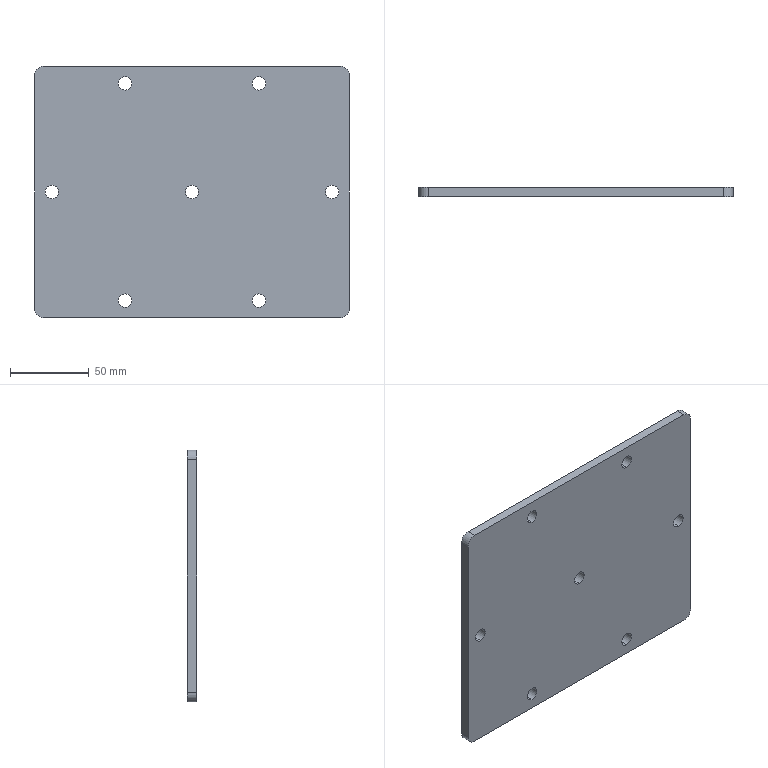Part | SolidWorks | features Extrusion 1, Fillet 1, HoleWzd 1 | 1 solid | 24 faces | box 200 x 6 x 160 mm | volume 189431 mm3 | cylinder 18 | plane 6 | commonest cylinder face diameters 8.5 x14 12 x4
STEP:
#1=CARTESIAN_POINT('',(0.,0.,-4.25));
#2=VERTEX_POINT('',#1);
#3=CARTESIAN_POINT('',(0.,0.,4.25));
#4=VERTEX_POINT('',#3);
#5=CARTESIAN_POINT('',(0.,0.,0.));
#6=DIRECTION('',(0.,1.,0.));
#7=DIRECTION('',(0.,0.,1.));
#8=AXIS2_PLACEMENT_3D('',#5,#6,#7);
#9=CIRCLE('',#8,4.25);
#10=EDGE_CURVE('',#2,#4,#9,.T.);
#11=ORIENTED_EDGE('',*,*,#10,.F.);
#12=CARTESIAN_POINT('',(0.,6.,-4.25));
#13=VERTEX_POINT('',#12);
#14=CARTESIAN_POINT('',(0.,6.,-4.25));
#15=DIRECTION('',(0.,1.,0.));
#16=VECTOR('',#15,1000.);
#17=LINE('',#14,#16);
#18=EDGE_CURVE('',#2,#13,#17,.T.);
#19=ORIENTED_EDGE('',*,*,#18,.T.);
#20=CARTESIAN_POINT('',(0.,6.,4.25));
#21=VERTEX_POINT('',#20);
#22=CARTESIAN_POINT('',(0.,6.,0.));
#23=DIRECTION('',(0.,1.,0.));
#24=DIRECTION('',(0.,0.,1.));
#25=AXIS2_PLACEMENT_3D('',#22,#23,#24);
#26=CIRCLE('',#25,4.25);
#27=EDGE_CURVE('',#13,#21,#26,.T.);
#28=ORIENTED_EDGE('',*,*,#27,.T.);
#29=CARTESIAN_POINT('',(0.,6.,4.25));
#30=DIRECTION('',(0.,1.,0.));
#31=VECTOR('',#30,1000.);
#32=LINE('',#29,#31);
#33=EDGE_CURVE('',#4,#21,#32,.T.);
#34=ORIENTED_EDGE('',*,*,#33,.F.);
#35=EDGE_LOOP('',(#11,#19,#28,#34));
#36=FACE_OUTER_BOUND('',#35,.T.);
#37=CARTESIAN_POINT('',(0.,6.,0.));
#38=DIRECTION('',(0.,1.,0.));
#39=DIRECTION('',(0.,0.,1.));
#40=AXIS2_PLACEMENT_3D('',#37,#38,#39);
#41=CYLINDRICAL_SURFACE('',#40,4.25);
#42=ADVANCED_FACE('',(#36),#41,.F.);
#43=CARTESIAN_POINT('',(42.5,0.,-73.25));
#44=VERTEX_POINT('',#43);
#45=CARTESIAN_POINT('',(42.5,0.,-64.75));
#46=VERTEX_POINT('',#45);
#47=CARTESIAN_POINT('',(42.5,0.,-69.));
#48=DIRECTION('',(0.,1.,0.));
#49=DIRECTION('',(0.,0.,1.));
#50=AXIS2_PLACEMENT_3D('',#47,#48,#49);
#51=CIRCLE('',#50,4.25);
#52=EDGE_CURVE('',#44,#46,#51,.T.);
#53=ORIENTED_EDGE('',*,*,#52,.F.);
#54=CARTESIAN_POINT('',(42.5,6.,-73.25));
#55=VERTEX_POINT('',#54);
#56=CARTESIAN_POINT('',(42.5,6.,-73.25));
#57=DIRECTION('',(0.,1.,0.));
#58=VECTOR('',#57,1000.);
#59=LINE('',#56,#58);
#60=EDGE_CURVE('',#44,#55,#59,.T.);
#61=ORIENTED_EDGE('',*,*,#60,.T.);
#62=CARTESIAN_POINT('',(42.5,6.,-64.75));
#63=VERTEX_POINT('',#62);
#64=CARTESIAN_POINT('',(42.5,6.,-69.));
#65=DIRECTION('',(0.,1.,0.));
#66=DIRECTION('',(0.,0.,1.));
#67=AXIS2_PLACEMENT_3D('',#64,#65,#66);
#68=CIRCLE('',#67,4.25);
#69=EDGE_CURVE('',#55,#63,#68,.T.);
#70=ORIENTED_EDGE('',*,*,#69,.T.);
#71=CARTESIAN_POINT('',(42.5,6.,-64.75));
#72=DIRECTION('',(0.,1.,0.));
#73=VECTOR('',#72,1000.);
#74=LINE('',#71,#73);
#75=EDGE_CURVE('',#46,#63,#74,.T.);
#76=ORIENTED_EDGE('',*,*,#75,.F.);
#77=EDGE_LOOP('',(#53,#61,#70,#76));
#78=FACE_OUTER_BOUND('',#77,.T.);
#79=CARTESIAN_POINT('',(42.5,6.,-69.));
#80=DIRECTION('',(0.,1.,0.));
#81=DIRECTION('',(0.,0.,1.));
#82=AXIS2_PLACEMENT_3D('',#79,#80,#81);
#83=CYLINDRICAL_SURFACE('',#82,4.25);
#84=ADVANCED_FACE('',(#78),#83,.F.);
#85=CARTESIAN_POINT('',(-42.5,0.,-73.25));
#86=VERTEX_POINT('',#85);
#87=CARTESIAN_POINT('',(-42.5,0.,-64.75));
#88=VERTEX_POINT('',#87);
#89=CARTESIAN_POINT('',(-42.5,0.,-69.));
#90=DIRECTION('',(0.,1.,0.));
#91=DIRECTION('',(0.,0.,1.));
#92=AXIS2_PLACEMENT_3D('',#89,#90,#91);
#93=CIRCLE('',#92,4.25);
#94=EDGE_CURVE('',#86,#88,#93,.T.);
#95=ORIENTED_EDGE('',*,*,#94,.F.);
#96=CARTESIAN_POINT('',(-42.5,6.,-73.25));
#97=VERTEX_POINT('',#96);
#98=CARTESIAN_POINT('',(-42.5,6.,-73.25));
#99=DIRECTION('',(0.,1.,0.));
#100=VECTOR('',#99,1000.);
#101=LINE('',#98,#100);
#102=EDGE_CURVE('',#86,#97,#101,.T.);
#103=ORIENTED_EDGE('',*,*,#102,.T.);
#104=CARTESIAN_POINT('',(-42.5,6.,-64.75));
#105=VERTEX_POINT('',#104);
#106=CARTESIAN_POINT('',(-42.5,6.,-69.));
#107=DIRECTION('',(0.,1.,0.));
#108=DIRECTION('',(0.,0.,1.));
#109=AXIS2_PLACEMENT_3D('',#106,#107,#108);
#110=CIRCLE('',#109,4.25);
#111=EDGE_CURVE('',#97,#105,#110,.T.);
#112=ORIENTED_EDGE('',*,*,#111,.T.);
#113=CARTESIAN_POINT('',(-42.5,6.,-64.75));
#114=DIRECTION('',(0.,1.,0.));
#115=VECTOR('',#114,1000.);
#116=LINE('',#113,#115);
#117=EDGE_CURVE('',#88,#105,#116,.T.);
#118=ORIENTED_EDGE('',*,*,#117,.F.);
#119=EDGE_LOOP('',(#95,#103,#112,#118));
#120=FACE_OUTER_BOUND('',#119,.T.);
#121=CARTESIAN_POINT('',(-42.5,6.,-69.));
#122=DIRECTION('',(0.,1.,0.));
#123=DIRECTION('',(0.,0.,1.));
#124=AXIS2_PLACEMENT_3D('',#121,#122,#123);
#125=CYLINDRICAL_SURFACE('',#124,4.25);
#126=ADVANCED_FACE('',(#120),#125,.F.);
#127=CARTESIAN_POINT('',(-89.,0.,-4.25));
#128=VERTEX_POINT('',#127);
#129=CARTESIAN_POINT('',(-89.,0.,4.25));
#130=VERTEX_POINT('',#129);
#131=CARTESIAN_POINT('',(-89.,0.,0.));
#132=DIRECTION('',(0.,1.,0.));
#133=DIRECTION('',(0.,0.,1.));
#134=AXIS2_PLACEMENT_3D('',#131,#132,#133);
#135=CIRCLE('',#134,4.25);
#136=EDGE_CURVE('',#128,#130,#135,.T.);
#137=ORIENTED_EDGE('',*,*,#136,.F.);
#138=CARTESIAN_POINT('',(-89.,6.,-4.25));
#139=VERTEX_POINT('',#138);
#140=CARTESIAN_POINT('',(-89.,6.,-4.25));
#141=DIRECTION('',(0.,1.,0.));
#142=VECTOR('',#141,1000.);
#143=LINE('',#140,#142);
#144=EDGE_CURVE('',#128,#139,#143,.T.);
#145=ORIENTED_EDGE('',*,*,#144,.T.);
#146=CARTESIAN_POINT('',(-89.,6.,4.25));
#147=VERTEX_POINT('',#146);
#148=CARTESIAN_POINT('',(-89.,6.,0.));
#149=DIRECTION('',(0.,1.,0.));
#150=DIRECTION('',(0.,0.,1.));
#151=AXIS2_PLACEMENT_3D('',#148,#149,#150);
#152=CIRCLE('',#151,4.25);
#153=EDGE_CURVE('',#139,#147,#152,.T.);
#154=ORIENTED_EDGE('',*,*,#153,.T.);
#155=CARTESIAN_POINT('',(-89.,6.,4.25));
#156=DIRECTION('',(0.,1.,0.));
#157=VECTOR('',#156,1000.);
#158=LINE('',#155,#157);
#159=EDGE_CURVE('',#130,#147,#158,.T.);
#160=ORIENTED_EDGE('',*,*,#159,.F.);
#161=EDGE_LOOP('',(#137,#145,#154,#160));
#162=FACE_OUTER_BOUND('',#161,.T.);
#163=CARTESIAN_POINT('',(-89.,6.,0.));
#164=DIRECTION('',(0.,1.,0.));
#165=DIRECTION('',(0.,0.,1.));
#166=AXIS2_PLACEMENT_3D('',#163,#164,#165);
#167=CYLINDRICAL_SURFACE('',#166,4.25);
#168=ADVANCED_FACE('',(#162),#167,.F.);
#169=CARTESIAN_POINT('',(89.,0.,-4.25));
#170=VERTEX_POINT('',#169);
#171=CARTESIAN_POINT('',(89.,0.,4.25));
#172=VERTEX_POINT('',#171);
#173=CARTESIAN_POINT('',(89.,0.,0.));
#174=DIRECTION('',(0.,1.,0.));
#175=DIRECTION('',(0.,0.,1.));
#176=AXIS2_PLACEMENT_3D('',#173,#174,#175);
#177=CIRCLE('',#176,4.25);
#178=EDGE_CURVE('',#170,#172,#177,.T.);
#179=ORIENTED_EDGE('',*,*,#178,.F.);
#180=CARTESIAN_POINT('',(89.,6.,-4.25));
#181=VERTEX_POINT('',#180);
#182=CARTESIAN_POINT('',(89.,6.,-4.25));
#183=DIRECTION('',(0.,1.,0.));
#184=VECTOR('',#183,1000.);
#185=LINE('',#182,#184);
#186=EDGE_CURVE('',#170,#181,#185,.T.);
#187=ORIENTED_EDGE('',*,*,#186,.T.);
#188=CARTESIAN_POINT('',(89.,6.,4.25));
#189=VERTEX_POINT('',#188);
#190=CARTESIAN_POINT('',(89.,6.,0.));
#191=DIRECTION('',(0.,1.,0.));
#192=DIRECTION('',(0.,0.,1.));
#193=AXIS2_PLACEMENT_3D('',#190,#191,#192);
#194=CIRCLE('',#193,4.25);
#195=EDGE_CURVE('',#181,#189,#194,.T.);
#196=ORIENTED_EDGE('',*,*,#195,.T.);
#197=CARTESIAN_POINT('',(89.,6.,4.25));
#198=DIRECTION('',(0.,1.,0.));
#199=VECTOR('',#198,1000.);
#200=LINE('',#197,#199);
#201=EDGE_CURVE('',#172,#189,#200,.T.);
#202=ORIENTED_EDGE('',*,*,#201,.F.);
#203=EDGE_LOOP('',(#179,#187,#196,#202));
#204=FACE_OUTER_BOUND('',#203,.T.);
#205=CARTESIAN_POINT('',(89.,6.,0.));
#206=DIRECTION('',(0.,1.,0.));
#207=DIRECTION('',(0.,0.,1.));
#208=AXIS2_PLACEMENT_3D('',#205,#206,#207);
#209=CYLINDRICAL_SURFACE('',#208,4.25);
#210=ADVANCED_FACE('',(#204),#209,.F.);
#211=CARTESIAN_POINT('',(42.5,0.,64.75));
#212=VERTEX_POINT('',#211);
#213=CARTESIAN_POINT('',(42.5,0.,73.25));
#214=VERTEX_POINT('',#213);
#215=CARTESIAN_POINT('',(42.5,0.,69.));
#216=DIRECTION('',(0.,1.,0.));
#217=DIRECTION('',(0.,0.,1.));
#218=AXIS2_PLACEMENT_3D('',#215,#216,#217);
#219=CIRCLE('',#218,4.25);
#220=EDGE_CURVE('',#212,#214,#219,.T.);
#221=ORIENTED_EDGE('',*,*,#220,.F.);
#222=CARTESIAN_POINT('',(42.5,6.,64.75));
#223=VERTEX_POINT('',#222);
#224=CARTESIAN_POINT('',(42.5,6.,64.75));
#225=DIRECTION('',(0.,1.,0.));
#226=VECTOR('',#225,1000.);
#227=LINE('',#224,#226);
#228=EDGE_CURVE('',#212,#223,#227,.T.);
#229=ORIENTED_EDGE('',*,*,#228,.T.);
#230=CARTESIAN_POINT('',(42.5,6.,73.25));
#231=VERTEX_POINT('',#230);
#232=CARTESIAN_POINT('',(42.5,6.,69.));
#233=DIRECTION('',(0.,1.,0.));
#234=DIRECTION('',(0.,0.,1.));
#235=AXIS2_PLACEMENT_3D('',#232,#233,#234);
#236=CIRCLE('',#235,4.25);
#237=EDGE_CURVE('',#223,#231,#236,.T.);
#238=ORIENTED_EDGE('',*,*,#237,.T.);
#239=CARTESIAN_POINT('',(42.5,6.,73.25));
#240=DIRECTION('',(0.,1.,0.));
#241=VECTOR('',#240,1000.);
#242=LINE('',#239,#241);
#243=EDGE_CURVE('',#214,#231,#242,.T.);
#244=ORIENTED_EDGE('',*,*,#243,.F.);
#245=EDGE_LOOP('',(#221,#229,#238,#244));
#246=FACE_OUTER_BOUND('',#245,.T.);
#247=CARTESIAN_POINT('',(42.5,6.,69.));
#248=DIRECTION('',(0.,1.,0.));
#249=DIRECTION('',(0.,0.,1.));
#250=AXIS2_PLACEMENT_3D('',#247,#248,#249);
#251=CYLINDRICAL_SURFACE('',#250,4.25);
#252=ADVANCED_FACE('',(#246),#251,.F.);
#253=CARTESIAN_POINT('',(-42.5,0.,64.75));
#254=VERTEX_POINT('',#253);
#255=CARTESIAN_POINT('',(-42.5,0.,73.25));
#256=VERTEX_POINT('',#255);
#257=CARTESIAN_POINT('',(-42.5,0.,69.));
#258=DIRECTION('',(0.,1.,0.));
#259=DIRECTION('',(0.,0.,1.));
#260=AXIS2_PLACEMENT_3D('',#257,#258,#259);
#261=CIRCLE('',#260,4.25);
#262=EDGE_CURVE('',#254,#256,#261,.T.);
#263=ORIENTED_EDGE('',*,*,#262,.F.);
#264=CARTESIAN_POINT('',(-42.5,6.,64.75));
#265=VERTEX_POINT('',#264);
#266=CARTESIAN_POINT('',(-42.5,6.,64.75));
#267=DIRECTION('',(0.,1.,0.));
#268=VECTOR('',#267,1000.);
#269=LINE('',#266,#268);
#270=EDGE_CURVE('',#254,#265,#269,.T.);
#271=ORIENTED_EDGE('',*,*,#270,.T.);
#272=CARTESIAN_POINT('',(-42.5,6.,73.25));
#273=VERTEX_POINT('',#272);
#274=CARTESIAN_POINT('',(-42.5,6.,69.));
#275=DIRECTION('',(0.,1.,0.));
#276=DIRECTION('',(0.,0.,1.));
#277=AXIS2_PLACEMENT_3D('',#274,#275,#276);
#278=CIRCLE('',#277,4.25);
#279=EDGE_CURVE('',#265,#273,#278,.T.);
#280=ORIENTED_EDGE('',*,*,#279,.T.);
#281=CARTESIAN_POINT('',(-42.5,6.,73.25));
#282=DIRECTION('',(0.,1.,0.));
#283=VECTOR('',#282,1000.);
#284=LINE('',#281,#283);
#285=EDGE_CURVE('',#256,#273,#284,.T.);
#286=ORIENTED_EDGE('',*,*,#285,.F.);
#287=EDGE_LOOP('',(#263,#271,#280,#286));
#288=FACE_OUTER_BOUND('',#287,.T.);
#289=CARTESIAN_POINT('',(-42.5,6.,69.));
#290=DIRECTION('',(0.,1.,0.));
#291=DIRECTION('',(0.,0.,1.));
#292=AXIS2_PLACEMENT_3D('',#289,#290,#291);
#293=CYLINDRICAL_SURFACE('',#292,4.25);
#294=ADVANCED_FACE('',(#288),#293,.F.);
#295=CARTESIAN_POINT('',(0.,0.,0.));
#296=DIRECTION('',(0.,1.,0.));
#297=DIRECTION('',(0.,0.,1.));
#298=AXIS2_PLACEMENT_3D('',#295,#296,#297);
#299=CIRCLE('',#298,4.25);
#300=EDGE_CURVE('',#4,#2,#299,.T.);
#301=ORIENTED_EDGE('',*,*,#300,.T.);
#302=ORIENTED_EDGE('',*,*,#10,.T.);
#303=EDGE_LOOP('',(#301,#302));
#304=FACE_BOUND('',#303,.T.);
#305=CARTESIAN_POINT('',(42.5,0.,-69.));
#306=DIRECTION('',(0.,1.,0.));
#307=DIRECTION('',(0.,0.,1.));
#308=AXIS2_PLACEMENT_3D('',#305,#306,#307);
#309=CIRCLE('',#308,4.25);
#310=EDGE_CURVE('',#46,#44,#309,.T.);
#311=ORIENTED_EDGE('',*,*,#310,.T.);
#312=ORIENTED_EDGE('',*,*,#52,.T.);
#313=EDGE_LOOP('',(#311,#312));
#314=FACE_BOUND('',#313,.T.);
#315=CARTESIAN_POINT('',(-42.5,0.,-69.));
#316=DIRECTION('',(0.,1.,0.));
#317=DIRECTION('',(0.,0.,1.));
#318=AXIS2_PLACEMENT_3D('',#315,#316,#317);
#319=CIRCLE('',#318,4.25);
#320=EDGE_CURVE('',#88,#86,#319,.T.);
#321=ORIENTED_EDGE('',*,*,#320,.T.);
#322=ORIENTED_EDGE('',*,*,#94,.T.);
#323=EDGE_LOOP('',(#321,#322));
#324=FACE_BOUND('',#323,.T.);
#325=CARTESIAN_POINT('',(-100.,0.,-74.));
#326=VERTEX_POINT('',#325);
#327=CARTESIAN_POINT('',(-100.,0.,74.));
#328=VERTEX_POINT('',#327);
#329=CARTESIAN_POINT('',(-100.,0.,80.));
#330=DIRECTION('',(0.,0.,1.));
#331=VECTOR('',#330,1000.);
#332=LINE('',#329,#331);
#333=EDGE_CURVE('',#326,#328,#332,.T.);
#334=ORIENTED_EDGE('',*,*,#333,.F.);
#335=CARTESIAN_POINT('',(-94.,0.,-80.));
#336=VERTEX_POINT('',#335);
#337=CARTESIAN_POINT('',(-94.,0.,-74.));
#338=DIRECTION('',(0.,-1.,0.));
#339=DIRECTION('',(0.,0.,-1.));
#340=AXIS2_PLACEMENT_3D('',#337,#338,#339);
#341=CIRCLE('',#340,6.);
#342=EDGE_CURVE('',#326,#336,#341,.T.);
#343=ORIENTED_EDGE('',*,*,#342,.T.);
#344=CARTESIAN_POINT('',(94.,0.,-80.));
#345=VERTEX_POINT('',#344);
#346=CARTESIAN_POINT('',(-100.,0.,-80.));
#347=DIRECTION('',(-1.,0.,0.));
#348=VECTOR('',#347,1000.);
#349=LINE('',#346,#348);
#350=EDGE_CURVE('',#345,#336,#349,.T.);
#351=ORIENTED_EDGE('',*,*,#350,.F.);
#352=CARTESIAN_POINT('',(100.,0.,-74.));
#353=VERTEX_POINT('',#352);
#354=CARTESIAN_POINT('',(94.,0.,-74.));
#355=DIRECTION('',(0.,-1.,0.));
#356=DIRECTION('',(0.,0.,-1.));
#357=AXIS2_PLACEMENT_3D('',#354,#355,#356);
#358=CIRCLE('',#357,6.);
#359=EDGE_CURVE('',#345,#353,#358,.T.);
#360=ORIENTED_EDGE('',*,*,#359,.T.);
#361=CARTESIAN_POINT('',(100.,0.,74.));
#362=VERTEX_POINT('',#361);
#363=CARTESIAN_POINT('',(100.,0.,80.));
#364=DIRECTION('',(0.,0.,-1.));
#365=VECTOR('',#364,1000.);
#366=LINE('',#363,#365);
#367=EDGE_CURVE('',#362,#353,#366,.T.);
#368=ORIENTED_EDGE('',*,*,#367,.F.);
#369=CARTESIAN_POINT('',(94.,0.,80.));
#370=VERTEX_POINT('',#369);
#371=CARTESIAN_POINT('',(94.,0.,74.));
#372=DIRECTION('',(0.,-1.,0.));
#373=DIRECTION('',(0.,0.,-1.));
#374=AXIS2_PLACEMENT_3D('',#371,#372,#373);
#375=CIRCLE('',#374,6.);
#376=EDGE_CURVE('',#362,#370,#375,.T.);
#377=ORIENTED_EDGE('',*,*,#376,.T.);
#378=CARTESIAN_POINT('',(-94.,0.,80.));
#379=VERTEX_POINT('',#378);
#380=CARTESIAN_POINT('',(-100.,0.,80.));
#381=DIRECTION('',(1.,0.,0.));
#382=VECTOR('',#381,1000.);
#383=LINE('',#380,#382);
#384=EDGE_CURVE('',#379,#370,#383,.T.);
#385=ORIENTED_EDGE('',*,*,#384,.F.);
#386=CARTESIAN_POINT('',(-94.,0.,74.));
#387=DIRECTION('',(0.,-1.,0.));
#388=DIRECTION('',(0.,0.,-1.));
#389=AXIS2_PLACEMENT_3D('',#386,#387,#388);
#390=CIRCLE('',#389,6.);
#391=EDGE_CURVE('',#379,#328,#390,.T.);
#392=ORIENTED_EDGE('',*,*,#391,.T.);
#393=EDGE_LOOP('',(#334,#343,#351,#360,#368,#377,#385,#392));
#394=FACE_OUTER_BOUND('',#393,.T.);
#395=CARTESIAN_POINT('',(-42.5,0.,69.));
#396=DIRECTION('',(0.,1.,0.));
#397=DIRECTION('',(0.,0.,1.));
#398=AXIS2_PLACEMENT_3D('',#395,#396,#397);
#399=CIRCLE('',#398,4.25);
#400=EDGE_CURVE('',#256,#254,#399,.T.);
#401=ORIENTED_EDGE('',*,*,#400,.T.);
#402=ORIENTED_EDGE('',*,*,#262,.T.);
#403=EDGE_LOOP('',(#401,#402));
#404=FACE_BOUND('',#403,.T.);
#405=CARTESIAN_POINT('',(42.5,0.,69.));
#406=DIRECTION('',(0.,1.,0.));
#407=DIRECTION('',(0.,0.,1.));
#408=AXIS2_PLACEMENT_3D('',#405,#406,#407);
#409=CIRCLE('',#408,4.25);
#410=EDGE_CURVE('',#214,#212,#409,.T.);
#411=ORIENTED_EDGE('',*,*,#410,.T.);
#412=ORIENTED_EDGE('',*,*,#220,.T.);
#413=EDGE_LOOP('',(#411,#412));
#414=FACE_BOUND('',#413,.T.);
#415=CARTESIAN_POINT('',(89.,0.,0.));
#416=DIRECTION('',(0.,1.,0.));
#417=DIRECTION('',(0.,0.,1.));
#418=AXIS2_PLACEMENT_3D('',#415,#416,#417);
#419=CIRCLE('',#418,4.25);
#420=EDGE_CURVE('',#172,#170,#419,.T.);
#421=ORIENTED_EDGE('',*,*,#420,.T.);
#422=ORIENTED_EDGE('',*,*,#178,.T.);
#423=EDGE_LOOP('',(#421,#422));
#424=FACE_BOUND('',#423,.T.);
#425=CARTESIAN_POINT('',(-89.,0.,0.));
#426=DIRECTION('',(0.,1.,0.));
#427=DIRECTION('',(0.,0.,1.));
#428=AXIS2_PLACEMENT_3D('',#425,#426,#427);
#429=CIRCLE('',#428,4.25);
#430=EDGE_CURVE('',#130,#128,#429,.T.);
#431=ORIENTED_EDGE('',*,*,#430,.T.);
#432=ORIENTED_EDGE('',*,*,#136,.T.);
#433=EDGE_LOOP('',(#431,#432));
#434=FACE_BOUND('',#433,.T.);
#435=CARTESIAN_POINT('',(0.,0.,0.));
#436=DIRECTION('',(0.,-1.,0.));
#437=DIRECTION('',(0.,0.,-1.));
#438=AXIS2_PLACEMENT_3D('',#435,#436,#437);
#439=PLANE('',#438);
#440=ADVANCED_FACE('',(#304,#314,#324,#394,#404,#414,#424,#434),#439,.T.);
#441=ORIENTED_EDGE('',*,*,#367,.T.);
#442=CARTESIAN_POINT('',(100.,6.,-74.));
#443=VERTEX_POINT('',#442);
#444=CARTESIAN_POINT('',(100.,6.,-74.));
#445=DIRECTION('',(0.,1.,0.));
#446=VECTOR('',#445,1000.);
#447=LINE('',#444,#446);
#448=EDGE_CURVE('',#353,#443,#447,.T.);
#449=ORIENTED_EDGE('',*,*,#448,.T.);
#450=CARTESIAN_POINT('',(100.,6.,74.));
#451=VERTEX_POINT('',#450);
#452=CARTESIAN_POINT('',(100.,6.,80.));
#453=DIRECTION('',(0.,0.,-1.));
#454=VECTOR('',#453,1000.);
#455=LINE('',#452,#454);
#456=EDGE_CURVE('',#451,#443,#455,.T.);
#457=ORIENTED_EDGE('',*,*,#456,.F.);
#458=CARTESIAN_POINT('',(100.,6.,74.));
#459=DIRECTION('',(0.,-1.,0.));
#460=VECTOR('',#459,1000.);
#461=LINE('',#458,#460);
#462=EDGE_CURVE('',#451,#362,#461,.T.);
#463=ORIENTED_EDGE('',*,*,#462,.T.);
#464=EDGE_LOOP('',(#441,#449,#457,#463));
#465=FACE_OUTER_BOUND('',#464,.T.);
#466=CARTESIAN_POINT('',(100.,6.,80.));
#467=DIRECTION('',(-1.,0.,0.));
#468=DIRECTION('',(0.,0.,1.));
#469=AXIS2_PLACEMENT_3D('',#466,#467,#468);
#470=PLANE('',#469);
#471=ADVANCED_FACE('',(#465),#470,.F.);
#472=ORIENTED_EDGE('',*,*,#350,.T.);
#473=CARTESIAN_POINT('',(-94.,6.,-80.));
#474=VERTEX_POINT('',#473);
#475=CARTESIAN_POINT('',(-94.,6.,-80.));
#476=DIRECTION('',(0.,1.,0.));
#477=VECTOR('',#476,1000.);
#478=LINE('',#475,#477);
#479=EDGE_CURVE('',#336,#474,#478,.T.);
#480=ORIENTED_EDGE('',*,*,#479,.T.);
#481=CARTESIAN_POINT('',(94.,6.,-80.));
#482=VERTEX_POINT('',#481);
#483=CARTESIAN_POINT('',(-100.,6.,-80.));
#484=DIRECTION('',(-1.,0.,0.));
#485=VECTOR('',#484,1000.);
#486=LINE('',#483,#485);
#487=EDGE_CURVE('',#482,#474,#486,.T.);
#488=ORIENTED_EDGE('',*,*,#487,.F.);
#489=CARTESIAN_POINT('',(94.,6.,-80.));
#490=DIRECTION('',(0.,-1.,0.));
#491=VECTOR('',#490,1000.);
#492=LINE('',#489,#491);
#493=EDGE_CURVE('',#482,#345,#492,.T.);
#494=ORIENTED_EDGE('',*,*,#493,.T.);
#495=EDGE_LOOP('',(#472,#480,#488,#494));
#496=FACE_OUTER_BOUND('',#495,.T.);
#497=CARTESIAN_POINT('',(-100.,6.,-80.));
#498=DIRECTION('',(0.,0.,1.));
#499=DIRECTION('',(1.,0.,0.));
#500=AXIS2_PLACEMENT_3D('',#497,#498,#499);
#501=PLANE('',#500);
#502=ADVANCED_FACE('',(#496),#501,.F.);
#503=CARTESIAN_POINT('',(-100.,6.,-74.));
#504=VERTEX_POINT('',#503);
#505=CARTESIAN_POINT('',(-100.,6.,74.));
#506=VERTEX_POINT('',#505);
#507=CARTESIAN_POINT('',(-100.,6.,80.));
#508=DIRECTION('',(0.,0.,1.));
#509=VECTOR('',#508,1000.);
#510=LINE('',#507,#509);
#511=EDGE_CURVE('',#504,#506,#510,.T.);
#512=ORIENTED_EDGE('',*,*,#511,.F.);
#513=CARTESIAN_POINT('',(-100.,6.,-74.));
#514=DIRECTION('',(0.,-1.,0.));
#515=VECTOR('',#514,1000.);
#516=LINE('',#513,#515);
#517=EDGE_CURVE('',#504,#326,#516,.T.);
#518=ORIENTED_EDGE('',*,*,#517,.T.);
#519=ORIENTED_EDGE('',*,*,#333,.T.);
#520=CARTESIAN_POINT('',(-100.,6.,74.));
#521=DIRECTION('',(0.,1.,0.));
#522=VECTOR('',#521,1000.);
#523=LINE('',#520,#522);
#524=EDGE_CURVE('',#328,#506,#523,.T.);
#525=ORIENTED_EDGE('',*,*,#524,.T.);
#526=EDGE_LOOP('',(#512,#518,#519,#525));
#527=FACE_OUTER_BOUND('',#526,.T.);
#528=CARTESIAN_POINT('',(-100.,6.,80.));
#529=DIRECTION('',(1.,0.,0.));
#530=DIRECTION('',(0.,0.,-1.));
#531=AXIS2_PLACEMENT_3D('',#528,#529,#530);
#532=PLANE('',#531);
#533=ADVANCED_FACE('',(#527),#532,.F.);
#534=ORIENTED_EDGE('',*,*,#384,.T.);
#535=CARTESIAN_POINT('',(94.,6.,80.));
#536=VERTEX_POINT('',#535);
#537=CARTESIAN_POINT('',(94.,6.,80.));
#538=DIRECTION('',(0.,1.,0.));
#539=VECTOR('',#538,1000.);
#540=LINE('',#537,#539);
#541=EDGE_CURVE('',#370,#536,#540,.T.);
#542=ORIENTED_EDGE('',*,*,#541,.T.);
#543=CARTESIAN_POINT('',(-94.,6.,80.));
#544=VERTEX_POINT('',#543);
#545=CARTESIAN_POINT('',(-100.,6.,80.));
#546=DIRECTION('',(1.,0.,0.));
#547=VECTOR('',#546,1000.);
#548=LINE('',#545,#547);
#549=EDGE_CURVE('',#544,#536,#548,.T.);
#550=ORIENTED_EDGE('',*,*,#549,.F.);
#551=CARTESIAN_POINT('',(-94.,6.,80.));
#552=DIRECTION('',(0.,-1.,0.));
#553=VECTOR('',#552,1000.);
#554=LINE('',#551,#553);
#555=EDGE_CURVE('',#544,#379,#554,.T.);
#556=ORIENTED_EDGE('',*,*,#555,.T.);
#557=EDGE_LOOP('',(#534,#542,#550,#556));
#558=FACE_OUTER_BOUND('',#557,.T.);
#559=CARTESIAN_POINT('',(-100.,6.,80.));
#560=DIRECTION('',(0.,0.,-1.));
#561=DIRECTION('',(-1.,0.,0.));
#562=AXIS2_PLACEMENT_3D('',#559,#560,#561);
#563=PLANE('',#562);
#564=ADVANCED_FACE('',(#558),#563,.F.);
#565=CARTESIAN_POINT('',(0.,6.,0.));
#566=DIRECTION('',(0.,1.,0.));
#567=DIRECTION('',(0.,0.,1.));
#568=AXIS2_PLACEMENT_3D('',#565,#566,#567);
#569=CIRCLE('',#568,4.25);
#570=EDGE_CURVE('',#21,#13,#569,.T.);
#571=ORIENTED_EDGE('',*,*,#570,.F.);
#572=ORIENTED_EDGE('',*,*,#27,.F.);
#573=EDGE_LOOP('',(#571,#572));
#574=FACE_BOUND('',#573,.T.);
#575=CARTESIAN_POINT('',(42.5,6.,-69.));
#576=DIRECTION('',(0.,1.,0.));
#577=DIRECTION('',(0.,0.,1.));
#578=AXIS2_PLACEMENT_3D('',#575,#576,#577);
#579=CIRCLE('',#578,4.25);
#580=EDGE_CURVE('',#63,#55,#579,.T.);
#581=ORIENTED_EDGE('',*,*,#580,.F.);
#582=ORIENTED_EDGE('',*,*,#69,.F.);
#583=EDGE_LOOP('',(#581,#582));
#584=FACE_BOUND('',#583,.T.);
#585=CARTESIAN_POINT('',(-42.5,6.,-69.));
#586=DIRECTION('',(0.,1.,0.));
#587=DIRECTION('',(0.,0.,1.));
#588=AXIS2_PLACEMENT_3D('',#585,#586,#587);
#589=CIRCLE('',#588,4.25);
#590=EDGE_CURVE('',#105,#97,#589,.T.);
#591=ORIENTED_EDGE('',*,*,#590,.F.);
#592=ORIENTED_EDGE('',*,*,#111,.F.);
#593=EDGE_LOOP('',(#591,#592));
#594=FACE_BOUND('',#593,.T.);
#595=CARTESIAN_POINT('',(-89.,6.,0.));
#596=DIRECTION('',(0.,1.,0.));
#597=DIRECTION('',(0.,0.,1.));
#598=AXIS2_PLACEMENT_3D('',#595,#596,#597);
#599=CIRCLE('',#598,4.25);
#600=EDGE_CURVE('',#147,#139,#599,.T.);
#601=ORIENTED_EDGE('',*,*,#600,.F.);
#602=ORIENTED_EDGE('',*,*,#153,.F.);
#603=EDGE_LOOP('',(#601,#602));
#604=FACE_BOUND('',#603,.T.);
#605=CARTESIAN_POINT('',(89.,6.,0.));
#606=DIRECTION('',(0.,1.,0.));
#607=DIRECTION('',(0.,0.,1.));
#608=AXIS2_PLACEMENT_3D('',#605,#606,#607);
#609=CIRCLE('',#608,4.25);
#610=EDGE_CURVE('',#189,#181,#609,.T.);
#611=ORIENTED_EDGE('',*,*,#610,.F.);
#612=ORIENTED_EDGE('',*,*,#195,.F.);
#613=EDGE_LOOP('',(#611,#612));
#614=FACE_BOUND('',#613,.T.);
#615=CARTESIAN_POINT('',(42.5,6.,69.));
#616=DIRECTION('',(0.,1.,0.));
#617=DIRECTION('',(0.,0.,1.));
#618=AXIS2_PLACEMENT_3D('',#615,#616,#617);
#619=CIRCLE('',#618,4.25);
#620=EDGE_CURVE('',#231,#223,#619,.T.);
#621=ORIENTED_EDGE('',*,*,#620,.F.);
#622=ORIENTED_EDGE('',*,*,#237,.F.);
#623=EDGE_LOOP('',(#621,#622));
#624=FACE_BOUND('',#623,.T.);
#625=CARTESIAN_POINT('',(-42.5,6.,69.));
#626=DIRECTION('',(0.,1.,0.));
#627=DIRECTION('',(0.,0.,1.));
#628=AXIS2_PLACEMENT_3D('',#625,#626,#627);
#629=CIRCLE('',#628,4.25);
#630=EDGE_CURVE('',#273,#265,#629,.T.);
#631=ORIENTED_EDGE('',*,*,#630,.F.);
#632=ORIENTED_EDGE('',*,*,#279,.F.);
#633=EDGE_LOOP('',(#631,#632));
#634=FACE_BOUND('',#633,.T.);
#635=ORIENTED_EDGE('',*,*,#487,.T.);
#636=CARTESIAN_POINT('',(-94.,6.,-74.));
#637=DIRECTION('',(0.,1.,0.));
#638=DIRECTION('',(0.,0.,-1.));
#639=AXIS2_PLACEMENT_3D('',#636,#637,#638);
#640=CIRCLE('',#639,6.);
#641=EDGE_CURVE('',#474,#504,#640,.T.);
#642=ORIENTED_EDGE('',*,*,#641,.T.);
#643=ORIENTED_EDGE('',*,*,#511,.T.);
#644=CARTESIAN_POINT('',(-94.,6.,74.));
#645=DIRECTION('',(0.,1.,0.));
#646=DIRECTION('',(0.,0.,-1.));
#647=AXIS2_PLACEMENT_3D('',#644,#645,#646);
#648=CIRCLE('',#647,6.);
#649=EDGE_CURVE('',#506,#544,#648,.T.);
#650=ORIENTED_EDGE('',*,*,#649,.T.);
#651=ORIENTED_EDGE('',*,*,#549,.T.);
#652=CARTESIAN_POINT('',(94.,6.,74.));
#653=DIRECTION('',(0.,1.,0.));
#654=DIRECTION('',(0.,0.,-1.));
#655=AXIS2_PLACEMENT_3D('',#652,#653,#654);
#656=CIRCLE('',#655,6.);
#657=EDGE_CURVE('',#536,#451,#656,.T.);
#658=ORIENTED_EDGE('',*,*,#657,.T.);
#659=ORIENTED_EDGE('',*,*,#456,.T.);
#660=CARTESIAN_POINT('',(94.,6.,-74.));
#661=DIRECTION('',(0.,1.,0.));
#662=DIRECTION('',(0.,0.,-1.));
#663=AXIS2_PLACEMENT_3D('',#660,#661,#662);
#664=CIRCLE('',#663,6.);
#665=EDGE_CURVE('',#443,#482,#664,.T.);
#666=ORIENTED_EDGE('',*,*,#665,.T.);
#667=EDGE_LOOP('',(#635,#642,#643,#650,#651,#658,#659,#666));
#668=FACE_OUTER_BOUND('',#667,.T.);
#669=CARTESIAN_POINT('',(0.,6.,0.));
#670=DIRECTION('',(0.,-1.,0.));
#671=DIRECTION('',(0.,0.,-1.));
#672=AXIS2_PLACEMENT_3D('',#669,#670,#671);
#673=PLANE('',#672);
#674=ADVANCED_FACE('',(#574,#584,#594,#604,#614,#624,#634,#668),#673,.F.);
#675=ORIENTED_EDGE('',*,*,#641,.F.);
#676=ORIENTED_EDGE('',*,*,#479,.F.);
#677=ORIENTED_EDGE('',*,*,#342,.F.);
#678=ORIENTED_EDGE('',*,*,#517,.F.);
#679=EDGE_LOOP('',(#675,#676,#677,#678));
#680=FACE_OUTER_BOUND('',#679,.T.);
#681=CARTESIAN_POINT('',(-94.,6.,-74.));
#682=DIRECTION('',(0.,-1.,0.));
#683=DIRECTION('',(0.,0.,-1.));
#684=AXIS2_PLACEMENT_3D('',#681,#682,#683);
#685=CYLINDRICAL_SURFACE('',#684,6.);
#686=ADVANCED_FACE('',(#680),#685,.T.);
#687=ORIENTED_EDGE('',*,*,#665,.F.);
#688=ORIENTED_EDGE('',*,*,#448,.F.);
#689=ORIENTED_EDGE('',*,*,#359,.F.);
#690=ORIENTED_EDGE('',*,*,#493,.F.);
#691=EDGE_LOOP('',(#687,#688,#689,#690));
#692=FACE_OUTER_BOUND('',#691,.T.);
#693=CARTESIAN_POINT('',(94.,6.,-74.));
#694=DIRECTION('',(0.,-1.,0.));
#695=DIRECTION('',(0.,0.,-1.));
#696=AXIS2_PLACEMENT_3D('',#693,#694,#695);
#697=CYLINDRICAL_SURFACE('',#696,6.);
#698=ADVANCED_FACE('',(#692),#697,.T.);
#699=ORIENTED_EDGE('',*,*,#657,.F.);
#700=ORIENTED_EDGE('',*,*,#541,.F.);
#701=ORIENTED_EDGE('',*,*,#376,.F.);
#702=ORIENTED_EDGE('',*,*,#462,.F.);
#703=EDGE_LOOP('',(#699,#700,#701,#702));
#704=FACE_OUTER_BOUND('',#703,.T.);
#705=CARTESIAN_POINT('',(94.,6.,74.));
#706=DIRECTION('',(0.,-1.,0.));
#707=DIRECTION('',(0.,0.,-1.));
#708=AXIS2_PLACEMENT_3D('',#705,#706,#707);
#709=CYLINDRICAL_SURFACE('',#708,6.);
#710=ADVANCED_FACE('',(#704),#709,.T.);
#711=ORIENTED_EDGE('',*,*,#649,.F.);
#712=ORIENTED_EDGE('',*,*,#524,.F.);
#713=ORIENTED_EDGE('',*,*,#391,.F.);
#714=ORIENTED_EDGE('',*,*,#555,.F.);
#715=EDGE_LOOP('',(#711,#712,#713,#714));
#716=FACE_OUTER_BOUND('',#715,.T.);
#717=CARTESIAN_POINT('',(-94.,6.,74.));
#718=DIRECTION('',(0.,-1.,0.));
#719=DIRECTION('',(0.,0.,-1.));
#720=AXIS2_PLACEMENT_3D('',#717,#718,#719);
#721=CYLINDRICAL_SURFACE('',#720,6.);
#722=ADVANCED_FACE('',(#716),#721,.T.);
#723=ORIENTED_EDGE('',*,*,#270,.F.);
#724=ORIENTED_EDGE('',*,*,#400,.F.);
#725=ORIENTED_EDGE('',*,*,#285,.T.);
#726=ORIENTED_EDGE('',*,*,#630,.T.);
#727=EDGE_LOOP('',(#723,#724,#725,#726));
#728=FACE_OUTER_BOUND('',#727,.T.);
#729=CARTESIAN_POINT('',(-42.5,6.,69.));
#730=DIRECTION('',(0.,1.,0.));
#731=DIRECTION('',(0.,0.,1.));
#732=AXIS2_PLACEMENT_3D('',#729,#730,#731);
#733=CYLINDRICAL_SURFACE('',#732,4.25);
#734=ADVANCED_FACE('',(#728),#733,.F.);
#735=ORIENTED_EDGE('',*,*,#228,.F.);
#736=ORIENTED_EDGE('',*,*,#410,.F.);
#737=ORIENTED_EDGE('',*,*,#243,.T.);
#738=ORIENTED_EDGE('',*,*,#620,.T.);
#739=EDGE_LOOP('',(#735,#736,#737,#738));
#740=FACE_OUTER_BOUND('',#739,.T.);
#741=CARTESIAN_POINT('',(42.5,6.,69.));
#742=DIRECTION('',(0.,1.,0.));
#743=DIRECTION('',(0.,0.,1.));
#744=AXIS2_PLACEMENT_3D('',#741,#742,#743);
#745=CYLINDRICAL_SURFACE('',#744,4.25);
#746=ADVANCED_FACE('',(#740),#745,.F.);
#747=ORIENTED_EDGE('',*,*,#186,.F.);
#748=ORIENTED_EDGE('',*,*,#420,.F.);
#749=ORIENTED_EDGE('',*,*,#201,.T.);
#750=ORIENTED_EDGE('',*,*,#610,.T.);
#751=EDGE_LOOP('',(#747,#748,#749,#750));
#752=FACE_OUTER_BOUND('',#751,.T.);
#753=CARTESIAN_POINT('',(89.,6.,0.));
#754=DIRECTION('',(0.,1.,0.));
#755=DIRECTION('',(0.,0.,1.));
#756=AXIS2_PLACEMENT_3D('',#753,#754,#755);
#757=CYLINDRICAL_SURFACE('',#756,4.25);
#758=ADVANCED_FACE('',(#752),#757,.F.);
#759=ORIENTED_EDGE('',*,*,#144,.F.);
#760=ORIENTED_EDGE('',*,*,#430,.F.);
#761=ORIENTED_EDGE('',*,*,#159,.T.);
#762=ORIENTED_EDGE('',*,*,#600,.T.);
#763=EDGE_LOOP('',(#759,#760,#761,#762));
#764=FACE_OUTER_BOUND('',#763,.T.);
#765=CARTESIAN_POINT('',(-89.,6.,0.));
#766=DIRECTION('',(0.,1.,0.));
#767=DIRECTION('',(0.,0.,1.));
#768=AXIS2_PLACEMENT_3D('',#765,#766,#767);
#769=CYLINDRICAL_SURFACE('',#768,4.25);
#770=ADVANCED_FACE('',(#764),#769,.F.);
#771=ORIENTED_EDGE('',*,*,#102,.F.);
#772=ORIENTED_EDGE('',*,*,#320,.F.);
#773=ORIENTED_EDGE('',*,*,#117,.T.);
#774=ORIENTED_EDGE('',*,*,#590,.T.);
#775=EDGE_LOOP('',(#771,#772,#773,#774));
#776=FACE_OUTER_BOUND('',#775,.T.);
#777=CARTESIAN_POINT('',(-42.5,6.,-69.));
#778=DIRECTION('',(0.,1.,0.));
#779=DIRECTION('',(0.,0.,1.));
#780=AXIS2_PLACEMENT_3D('',#777,#778,#779);
#781=CYLINDRICAL_SURFACE('',#780,4.25);
#782=ADVANCED_FACE('',(#776),#781,.F.);
#783=ORIENTED_EDGE('',*,*,#60,.F.);
#784=ORIENTED_EDGE('',*,*,#310,.F.);
#785=ORIENTED_EDGE('',*,*,#75,.T.);
#786=ORIENTED_EDGE('',*,*,#580,.T.);
#787=EDGE_LOOP('',(#783,#784,#785,#786));
#788=FACE_OUTER_BOUND('',#787,.T.);
#789=CARTESIAN_POINT('',(42.5,6.,-69.));
#790=DIRECTION('',(0.,1.,0.));
#791=DIRECTION('',(0.,0.,1.));
#792=AXIS2_PLACEMENT_3D('',#789,#790,#791);
#793=CYLINDRICAL_SURFACE('',#792,4.25);
#794=ADVANCED_FACE('',(#788),#793,.F.);
#795=ORIENTED_EDGE('',*,*,#18,.F.);
#796=ORIENTED_EDGE('',*,*,#300,.F.);
#797=ORIENTED_EDGE('',*,*,#33,.T.);
#798=ORIENTED_EDGE('',*,*,#570,.T.);
#799=EDGE_LOOP('',(#795,#796,#797,#798));
#800=FACE_OUTER_BOUND('',#799,.T.);
#801=CARTESIAN_POINT('',(0.,6.,0.));
#802=DIRECTION('',(0.,1.,0.));
#803=DIRECTION('',(0.,0.,1.));
#804=AXIS2_PLACEMENT_3D('',#801,#802,#803);
#805=CYLINDRICAL_SURFACE('',#804,4.25);
#806=ADVANCED_FACE('',(#800),#805,.F.);
#807=CLOSED_SHELL('',(#42,#84,#126,#168,#210,#252,#294,#440,#471,#502,#533,#564,#674,#686,#698,#710,#722,#734,#746,#758,#770,#782,#794,#806));
#808=MANIFOLD_SOLID_BREP('',#807);
#809=CARTESIAN_POINT('',(0.,0.,0.));
#810=DIRECTION('',(0.,0.,1.));
#811=DIRECTION('',(1.,0.,0.));
#812=AXIS2_PLACEMENT_3D('',#809,#810,#811);
#813=(LENGTH_UNIT()NAMED_UNIT(*)SI_UNIT(.MILLI.,.METRE.));
#814=UNCERTAINTY_MEASURE_WITH_UNIT(LENGTH_MEASURE(0.00001),#813,'','');
#815=(NAMED_UNIT(*)PLANE_ANGLE_UNIT()SI_UNIT($,.RADIAN.));
#816=(NAMED_UNIT(*)SI_UNIT($,.STERADIAN.)SOLID_ANGLE_UNIT());
#817=(GEOMETRIC_REPRESENTATION_CONTEXT(3)GLOBAL_UNCERTAINTY_ASSIGNED_CONTEXT((#814))GLOBAL_UNIT_ASSIGNED_CONTEXT((#813,#815,#816))REPRESENTATION_CONTEXT('',''));
#818=ADVANCED_BREP_SHAPE_REPRESENTATION('',(#808,#812),#817);